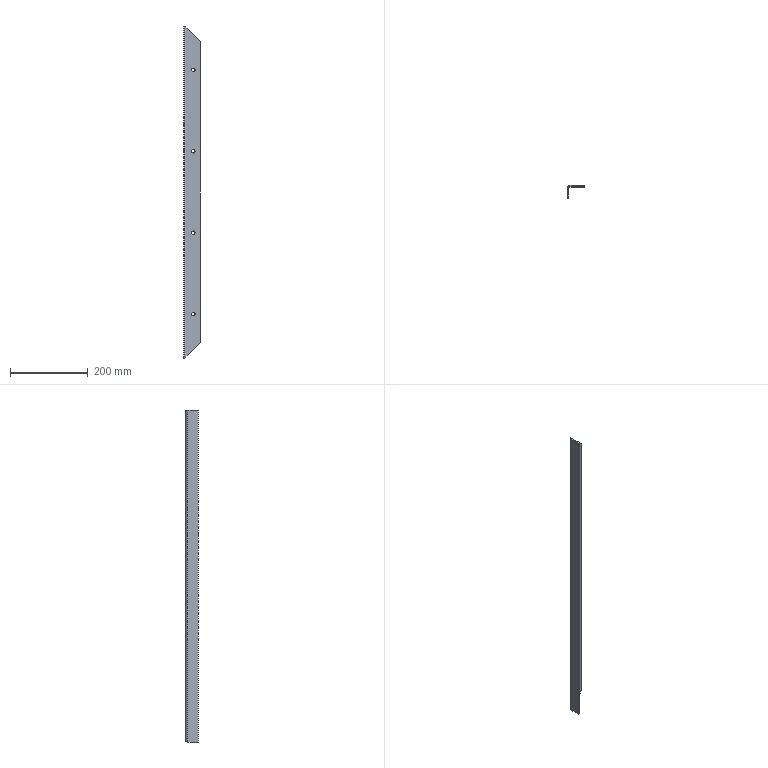Part | STEP file | 750038392 | 1 solid | 22 faces | box 43 x 33 x 856 mm | volume 176921 mm3 | cylinder 10 | plane 10 | spline 2 | commonest cylinder face diameters 9 x8 6 x1 12 x1
STEP:
#1=CARTESIAN_POINT('',(22.,0.,310.5));
#2=VERTEX_POINT('',#1);
#3=CARTESIAN_POINT('',(22.,0.,319.5));
#4=VERTEX_POINT('',#3);
#5=CARTESIAN_POINT('',(22.,0.,315.));
#6=DIRECTION('',(0.,1.,0.));
#7=DIRECTION('',(0.,0.,1.));
#8=AXIS2_PLACEMENT_3D('',#5,#6,#7);
#9=CIRCLE('',#8,4.5);
#10=EDGE_CURVE('',#2,#4,#9,.T.);
#11=ORIENTED_EDGE('',*,*,#10,.F.);
#12=CARTESIAN_POINT('',(22.,3.,310.5));
#13=VERTEX_POINT('',#12);
#14=CARTESIAN_POINT('',(22.,-854.714,310.5));
#15=DIRECTION('',(0.,1.,0.));
#16=VECTOR('',#15,1000.);
#17=LINE('',#14,#16);
#18=EDGE_CURVE('',#2,#13,#17,.T.);
#19=ORIENTED_EDGE('',*,*,#18,.T.);
#20=CARTESIAN_POINT('',(22.,3.,319.5));
#21=VERTEX_POINT('',#20);
#22=CARTESIAN_POINT('',(22.,3.,315.));
#23=DIRECTION('',(0.,1.,0.));
#24=DIRECTION('',(0.,0.,1.));
#25=AXIS2_PLACEMENT_3D('',#22,#23,#24);
#26=CIRCLE('',#25,4.5);
#27=EDGE_CURVE('',#13,#21,#26,.T.);
#28=ORIENTED_EDGE('',*,*,#27,.T.);
#29=CARTESIAN_POINT('',(22.,-854.714,319.5));
#30=DIRECTION('',(0.,1.,0.));
#31=VECTOR('',#30,1000.);
#32=LINE('',#29,#31);
#33=EDGE_CURVE('',#4,#21,#32,.T.);
#34=ORIENTED_EDGE('',*,*,#33,.F.);
#35=EDGE_LOOP('',(#11,#19,#28,#34));
#36=FACE_OUTER_BOUND('',#35,.T.);
#37=CARTESIAN_POINT('',(22.,-854.714,315.));
#38=DIRECTION('',(0.,1.,0.));
#39=DIRECTION('',(0.,0.,1.));
#40=AXIS2_PLACEMENT_3D('',#37,#38,#39);
#41=CYLINDRICAL_SURFACE('',#40,4.5);
#42=ADVANCED_FACE('',(#36),#41,.F.);
#43=CARTESIAN_POINT('',(22.,0.,100.5));
#44=VERTEX_POINT('',#43);
#45=CARTESIAN_POINT('',(22.,0.,109.5));
#46=VERTEX_POINT('',#45);
#47=CARTESIAN_POINT('',(22.,0.,105.));
#48=DIRECTION('',(0.,1.,0.));
#49=DIRECTION('',(0.,0.,1.));
#50=AXIS2_PLACEMENT_3D('',#47,#48,#49);
#51=CIRCLE('',#50,4.5);
#52=EDGE_CURVE('',#44,#46,#51,.T.);
#53=ORIENTED_EDGE('',*,*,#52,.F.);
#54=CARTESIAN_POINT('',(22.,3.,100.5));
#55=VERTEX_POINT('',#54);
#56=CARTESIAN_POINT('',(22.,-854.714,100.5));
#57=DIRECTION('',(0.,1.,0.));
#58=VECTOR('',#57,1000.);
#59=LINE('',#56,#58);
#60=EDGE_CURVE('',#44,#55,#59,.T.);
#61=ORIENTED_EDGE('',*,*,#60,.T.);
#62=CARTESIAN_POINT('',(22.,3.,109.5));
#63=VERTEX_POINT('',#62);
#64=CARTESIAN_POINT('',(22.,3.,105.));
#65=DIRECTION('',(0.,1.,0.));
#66=DIRECTION('',(0.,0.,1.));
#67=AXIS2_PLACEMENT_3D('',#64,#65,#66);
#68=CIRCLE('',#67,4.5);
#69=EDGE_CURVE('',#55,#63,#68,.T.);
#70=ORIENTED_EDGE('',*,*,#69,.T.);
#71=CARTESIAN_POINT('',(22.,-854.714,109.5));
#72=DIRECTION('',(0.,1.,0.));
#73=VECTOR('',#72,1000.);
#74=LINE('',#71,#73);
#75=EDGE_CURVE('',#46,#63,#74,.T.);
#76=ORIENTED_EDGE('',*,*,#75,.F.);
#77=EDGE_LOOP('',(#53,#61,#70,#76));
#78=FACE_OUTER_BOUND('',#77,.T.);
#79=CARTESIAN_POINT('',(22.,-854.714,105.));
#80=DIRECTION('',(0.,1.,0.));
#81=DIRECTION('',(0.,0.,1.));
#82=AXIS2_PLACEMENT_3D('',#79,#80,#81);
#83=CYLINDRICAL_SURFACE('',#82,4.5);
#84=ADVANCED_FACE('',(#78),#83,.F.);
#85=CARTESIAN_POINT('',(22.,0.,-109.5));
#86=VERTEX_POINT('',#85);
#87=CARTESIAN_POINT('',(22.,0.,-100.5));
#88=VERTEX_POINT('',#87);
#89=CARTESIAN_POINT('',(22.,0.,-105.));
#90=DIRECTION('',(0.,1.,0.));
#91=DIRECTION('',(0.,0.,1.));
#92=AXIS2_PLACEMENT_3D('',#89,#90,#91);
#93=CIRCLE('',#92,4.5);
#94=EDGE_CURVE('',#86,#88,#93,.T.);
#95=ORIENTED_EDGE('',*,*,#94,.F.);
#96=CARTESIAN_POINT('',(22.,3.,-109.5));
#97=VERTEX_POINT('',#96);
#98=CARTESIAN_POINT('',(22.,-854.714,-109.5));
#99=DIRECTION('',(0.,1.,0.));
#100=VECTOR('',#99,1000.);
#101=LINE('',#98,#100);
#102=EDGE_CURVE('',#86,#97,#101,.T.);
#103=ORIENTED_EDGE('',*,*,#102,.T.);
#104=CARTESIAN_POINT('',(22.,3.,-100.5));
#105=VERTEX_POINT('',#104);
#106=CARTESIAN_POINT('',(22.,3.,-105.));
#107=DIRECTION('',(0.,1.,0.));
#108=DIRECTION('',(0.,0.,1.));
#109=AXIS2_PLACEMENT_3D('',#106,#107,#108);
#110=CIRCLE('',#109,4.5);
#111=EDGE_CURVE('',#97,#105,#110,.T.);
#112=ORIENTED_EDGE('',*,*,#111,.T.);
#113=CARTESIAN_POINT('',(22.,-854.714,-100.5));
#114=DIRECTION('',(0.,1.,0.));
#115=VECTOR('',#114,1000.);
#116=LINE('',#113,#115);
#117=EDGE_CURVE('',#88,#105,#116,.T.);
#118=ORIENTED_EDGE('',*,*,#117,.F.);
#119=EDGE_LOOP('',(#95,#103,#112,#118));
#120=FACE_OUTER_BOUND('',#119,.T.);
#121=CARTESIAN_POINT('',(22.,-854.714,-105.));
#122=DIRECTION('',(0.,1.,0.));
#123=DIRECTION('',(0.,0.,1.));
#124=AXIS2_PLACEMENT_3D('',#121,#122,#123);
#125=CYLINDRICAL_SURFACE('',#124,4.5);
#126=ADVANCED_FACE('',(#120),#125,.F.);
#127=CARTESIAN_POINT('',(22.,0.,-319.5));
#128=VERTEX_POINT('',#127);
#129=CARTESIAN_POINT('',(22.,0.,-310.5));
#130=VERTEX_POINT('',#129);
#131=CARTESIAN_POINT('',(22.,0.,-315.));
#132=DIRECTION('',(0.,1.,0.));
#133=DIRECTION('',(0.,0.,1.));
#134=AXIS2_PLACEMENT_3D('',#131,#132,#133);
#135=CIRCLE('',#134,4.5);
#136=EDGE_CURVE('',#128,#130,#135,.T.);
#137=ORIENTED_EDGE('',*,*,#136,.F.);
#138=CARTESIAN_POINT('',(22.,3.,-319.5));
#139=VERTEX_POINT('',#138);
#140=CARTESIAN_POINT('',(22.,-854.714,-319.5));
#141=DIRECTION('',(0.,1.,0.));
#142=VECTOR('',#141,1000.);
#143=LINE('',#140,#142);
#144=EDGE_CURVE('',#128,#139,#143,.T.);
#145=ORIENTED_EDGE('',*,*,#144,.T.);
#146=CARTESIAN_POINT('',(22.,3.,-310.5));
#147=VERTEX_POINT('',#146);
#148=CARTESIAN_POINT('',(22.,3.,-315.));
#149=DIRECTION('',(0.,1.,0.));
#150=DIRECTION('',(0.,0.,1.));
#151=AXIS2_PLACEMENT_3D('',#148,#149,#150);
#152=CIRCLE('',#151,4.5);
#153=EDGE_CURVE('',#139,#147,#152,.T.);
#154=ORIENTED_EDGE('',*,*,#153,.T.);
#155=CARTESIAN_POINT('',(22.,-854.714,-310.5));
#156=DIRECTION('',(0.,1.,0.));
#157=VECTOR('',#156,1000.);
#158=LINE('',#155,#157);
#159=EDGE_CURVE('',#130,#147,#158,.T.);
#160=ORIENTED_EDGE('',*,*,#159,.F.);
#161=EDGE_LOOP('',(#137,#145,#154,#160));
#162=FACE_OUTER_BOUND('',#161,.T.);
#163=CARTESIAN_POINT('',(22.,-854.714,-315.));
#164=DIRECTION('',(0.,1.,0.));
#165=DIRECTION('',(0.,0.,1.));
#166=AXIS2_PLACEMENT_3D('',#163,#164,#165);
#167=CYLINDRICAL_SURFACE('',#166,4.5);
#168=ADVANCED_FACE('',(#162),#167,.F.);
#169=CARTESIAN_POINT('',(40.,3.,-388.));
#170=VERTEX_POINT('',#169);
#171=CARTESIAN_POINT('',(40.,3.,388.));
#172=VERTEX_POINT('',#171);
#173=CARTESIAN_POINT('',(40.,3.,428.));
#174=DIRECTION('',(0.,0.,1.));
#175=VECTOR('',#174,1000.);
#176=LINE('',#173,#175);
#177=EDGE_CURVE('',#170,#172,#176,.T.);
#178=ORIENTED_EDGE('',*,*,#177,.F.);
#179=CARTESIAN_POINT('',(3.,3.,-425.));
#180=VERTEX_POINT('',#179);
#181=CARTESIAN_POINT('',(3.,3.,-425.));
#182=DIRECTION('',(0.7071,0.,0.7071));
#183=VECTOR('',#182,1000.);
#184=LINE('',#181,#183);
#185=EDGE_CURVE('',#180,#170,#184,.T.);
#186=ORIENTED_EDGE('',*,*,#185,.F.);
#187=CARTESIAN_POINT('',(3.,3.,425.));
#188=VERTEX_POINT('',#187);
#189=CARTESIAN_POINT('',(3.,3.,428.));
#190=DIRECTION('',(0.,0.,-1.));
#191=VECTOR('',#190,1000.);
#192=LINE('',#189,#191);
#193=EDGE_CURVE('',#188,#180,#192,.T.);
#194=ORIENTED_EDGE('',*,*,#193,.F.);
#195=CARTESIAN_POINT('',(40.,3.,388.));
#196=DIRECTION('',(-0.7071,0.,0.7071));
#197=VECTOR('',#196,1000.);
#198=LINE('',#195,#197);
#199=EDGE_CURVE('',#172,#188,#198,.T.);
#200=ORIENTED_EDGE('',*,*,#199,.F.);
#201=EDGE_LOOP('',(#178,#186,#194,#200));
#202=FACE_OUTER_BOUND('',#201,.T.);
#203=CARTESIAN_POINT('',(22.,3.,315.));
#204=DIRECTION('',(0.,1.,0.));
#205=DIRECTION('',(0.,0.,1.));
#206=AXIS2_PLACEMENT_3D('',#203,#204,#205);
#207=CIRCLE('',#206,4.5);
#208=EDGE_CURVE('',#21,#13,#207,.T.);
#209=ORIENTED_EDGE('',*,*,#208,.F.);
#210=ORIENTED_EDGE('',*,*,#27,.F.);
#211=EDGE_LOOP('',(#209,#210));
#212=FACE_BOUND('',#211,.T.);
#213=CARTESIAN_POINT('',(22.,3.,105.));
#214=DIRECTION('',(0.,1.,0.));
#215=DIRECTION('',(0.,0.,1.));
#216=AXIS2_PLACEMENT_3D('',#213,#214,#215);
#217=CIRCLE('',#216,4.5);
#218=EDGE_CURVE('',#63,#55,#217,.T.);
#219=ORIENTED_EDGE('',*,*,#218,.F.);
#220=ORIENTED_EDGE('',*,*,#69,.F.);
#221=EDGE_LOOP('',(#219,#220));
#222=FACE_BOUND('',#221,.T.);
#223=CARTESIAN_POINT('',(22.,3.,-105.));
#224=DIRECTION('',(0.,1.,0.));
#225=DIRECTION('',(0.,0.,1.));
#226=AXIS2_PLACEMENT_3D('',#223,#224,#225);
#227=CIRCLE('',#226,4.5);
#228=EDGE_CURVE('',#105,#97,#227,.T.);
#229=ORIENTED_EDGE('',*,*,#228,.F.);
#230=ORIENTED_EDGE('',*,*,#111,.F.);
#231=EDGE_LOOP('',(#229,#230));
#232=FACE_BOUND('',#231,.T.);
#233=CARTESIAN_POINT('',(22.,3.,-315.));
#234=DIRECTION('',(0.,1.,0.));
#235=DIRECTION('',(0.,0.,1.));
#236=AXIS2_PLACEMENT_3D('',#233,#234,#235);
#237=CIRCLE('',#236,4.5);
#238=EDGE_CURVE('',#147,#139,#237,.T.);
#239=ORIENTED_EDGE('',*,*,#238,.F.);
#240=ORIENTED_EDGE('',*,*,#153,.F.);
#241=EDGE_LOOP('',(#239,#240));
#242=FACE_BOUND('',#241,.T.);
#243=CARTESIAN_POINT('',(40.,3.,428.));
#244=DIRECTION('',(0.,-1.,0.));
#245=DIRECTION('',(0.,0.,-1.));
#246=AXIS2_PLACEMENT_3D('',#243,#244,#245);
#247=PLANE('',#246);
#248=ADVANCED_FACE('',(#202,#212,#222,#232,#242),#247,.F.);
#249=CARTESIAN_POINT('',(40.,0.,388.));
#250=VERTEX_POINT('',#249);
#251=CARTESIAN_POINT('',(40.,0.,388.));
#252=DIRECTION('',(0.,1.,0.));
#253=VECTOR('',#252,1000.);
#254=LINE('',#251,#253);
#255=EDGE_CURVE('',#250,#172,#254,.T.);
#256=ORIENTED_EDGE('',*,*,#255,.T.);
#257=ORIENTED_EDGE('',*,*,#199,.T.);
#258=CARTESIAN_POINT('',(3.,0.,425.));
#259=VERTEX_POINT('',#258);
#260=CARTESIAN_POINT('',(3.,0.,425.));
#261=DIRECTION('',(0.,-1.,0.));
#262=VECTOR('',#261,1000.);
#263=LINE('',#260,#262);
#264=EDGE_CURVE('',#188,#259,#263,.T.);
#265=ORIENTED_EDGE('',*,*,#264,.T.);
#266=CARTESIAN_POINT('',(20.,0.,408.));
#267=DIRECTION('',(0.7071,0.,-0.7071));
#268=VECTOR('',#267,1000.);
#269=LINE('',#266,#268);
#270=EDGE_CURVE('',#259,#250,#269,.T.);
#271=ORIENTED_EDGE('',*,*,#270,.T.);
#272=EDGE_LOOP('',(#256,#257,#265,#271));
#273=FACE_OUTER_BOUND('',#272,.T.);
#274=CARTESIAN_POINT('',(20.,0.,408.));
#275=DIRECTION('',(0.7071,0.,0.7071));
#276=DIRECTION('',(0.7071,0.,-0.7071));
#277=AXIS2_PLACEMENT_3D('',#274,#275,#276);
#278=PLANE('',#277);
#279=ADVANCED_FACE('',(#273),#278,.T.);
#280=ORIENTED_EDGE('',*,*,#255,.F.);
#281=CARTESIAN_POINT('',(40.,0.,-388.));
#282=VERTEX_POINT('',#281);
#283=CARTESIAN_POINT('',(40.,0.,428.));
#284=DIRECTION('',(0.,0.,1.));
#285=VECTOR('',#284,1000.);
#286=LINE('',#283,#285);
#287=EDGE_CURVE('',#282,#250,#286,.T.);
#288=ORIENTED_EDGE('',*,*,#287,.F.);
#289=CARTESIAN_POINT('',(40.,0.,-388.));
#290=DIRECTION('',(0.,-1.,0.));
#291=VECTOR('',#290,1000.);
#292=LINE('',#289,#291);
#293=EDGE_CURVE('',#170,#282,#292,.T.);
#294=ORIENTED_EDGE('',*,*,#293,.F.);
#295=ORIENTED_EDGE('',*,*,#177,.T.);
#296=EDGE_LOOP('',(#280,#288,#294,#295));
#297=FACE_OUTER_BOUND('',#296,.T.);
#298=CARTESIAN_POINT('',(40.,0.,428.));
#299=DIRECTION('',(-1.,0.,0.));
#300=DIRECTION('',(0.,0.,1.));
#301=AXIS2_PLACEMENT_3D('',#298,#299,#300);
#302=PLANE('',#301);
#303=ADVANCED_FACE('',(#297),#302,.F.);
#304=CARTESIAN_POINT('',(3.,0.,-425.));
#305=VERTEX_POINT('',#304);
#306=CARTESIAN_POINT('',(3.,0.,-425.));
#307=DIRECTION('',(0.,1.,0.));
#308=VECTOR('',#307,1000.);
#309=LINE('',#306,#308);
#310=EDGE_CURVE('',#305,#180,#309,.T.);
#311=ORIENTED_EDGE('',*,*,#310,.T.);
#312=ORIENTED_EDGE('',*,*,#185,.T.);
#313=ORIENTED_EDGE('',*,*,#293,.T.);
#314=CARTESIAN_POINT('',(448.,0.,20.));
#315=DIRECTION('',(-0.7071,0.,-0.7071));
#316=VECTOR('',#315,1000.);
#317=LINE('',#314,#316);
#318=EDGE_CURVE('',#282,#305,#317,.T.);
#319=ORIENTED_EDGE('',*,*,#318,.T.);
#320=EDGE_LOOP('',(#311,#312,#313,#319));
#321=FACE_OUTER_BOUND('',#320,.T.);
#322=CARTESIAN_POINT('',(448.,0.,20.));
#323=DIRECTION('',(0.7071,0.,-0.7071));
#324=DIRECTION('',(-0.7071,0.,-0.7071));
#325=AXIS2_PLACEMENT_3D('',#322,#323,#324);
#326=PLANE('',#325);
#327=ADVANCED_FACE('',(#321),#326,.T.);
#328=CARTESIAN_POINT('',(-3.,-3.,-428.));
#329=VERTEX_POINT('',#328);
#330=CARTESIAN_POINT('',(3.,3.,-425.));
#331=CARTESIAN_POINT('',(-1.,3.,-427.));
#332=CARTESIAN_POINT('',(-3.,0.,-428.));
#333=CARTESIAN_POINT('',(-3.,-3.,-428.));
#334=(BOUNDED_CURVE()B_SPLINE_CURVE(3,(#330,#331,#332,#333),.UNSPECIFIED.,.F.,.F.)B_SPLINE_CURVE_WITH_KNOTS((4,4),(0.,0.009933),.UNSPECIFIED.)CURVE()GEOMETRIC_REPRESENTATION_ITEM()RATIONAL_B_SPLINE_CURVE((0.5,0.5,0.6667,1.))REPRESENTATION_ITEM(''));
#335=EDGE_CURVE('',#180,#329,#334,.T.);
#336=ORIENTED_EDGE('',*,*,#335,.T.);
#337=CARTESIAN_POINT('',(-3.,-3.,428.));
#338=VERTEX_POINT('',#337);
#339=CARTESIAN_POINT('',(-3.,-3.,428.));
#340=DIRECTION('',(0.,0.,1.));
#341=VECTOR('',#340,1000.);
#342=LINE('',#339,#341);
#343=EDGE_CURVE('',#329,#338,#342,.T.);
#344=ORIENTED_EDGE('',*,*,#343,.T.);
#345=CARTESIAN_POINT('',(-3.,-3.,428.));
#346=CARTESIAN_POINT('',(-3.,0.,428.));
#347=CARTESIAN_POINT('',(-1.,3.,427.));
#348=CARTESIAN_POINT('',(3.,3.,425.));
#349=(BOUNDED_CURVE()B_SPLINE_CURVE(3,(#345,#346,#347,#348),.UNSPECIFIED.,.F.,.T.)B_SPLINE_CURVE_WITH_KNOTS((4,4),(0.,0.009979),.UNSPECIFIED.)CURVE()GEOMETRIC_REPRESENTATION_ITEM()RATIONAL_B_SPLINE_CURVE((1.,0.6667,0.5,0.5))REPRESENTATION_ITEM(''));
#350=EDGE_CURVE('',#338,#188,#349,.T.);
#351=ORIENTED_EDGE('',*,*,#350,.T.);
#352=ORIENTED_EDGE('',*,*,#193,.T.);
#353=EDGE_LOOP('',(#336,#344,#351,#352));
#354=FACE_OUTER_BOUND('',#353,.T.);
#355=CARTESIAN_POINT('',(3.,-3.,428.));
#356=DIRECTION('',(0.,0.,-1.));
#357=DIRECTION('',(-1.,0.,0.));
#358=AXIS2_PLACEMENT_3D('',#355,#356,#357);
#359=CYLINDRICAL_SURFACE('',#358,6.);
#360=ADVANCED_FACE('',(#354),#359,.T.);
#361=ORIENTED_EDGE('',*,*,#18,.F.);
#362=CARTESIAN_POINT('',(22.,0.,315.));
#363=DIRECTION('',(0.,1.,0.));
#364=DIRECTION('',(0.,0.,1.));
#365=AXIS2_PLACEMENT_3D('',#362,#363,#364);
#366=CIRCLE('',#365,4.5);
#367=EDGE_CURVE('',#4,#2,#366,.T.);
#368=ORIENTED_EDGE('',*,*,#367,.F.);
#369=ORIENTED_EDGE('',*,*,#33,.T.);
#370=ORIENTED_EDGE('',*,*,#208,.T.);
#371=EDGE_LOOP('',(#361,#368,#369,#370));
#372=FACE_OUTER_BOUND('',#371,.T.);
#373=CARTESIAN_POINT('',(22.,-854.714,315.));
#374=DIRECTION('',(0.,1.,0.));
#375=DIRECTION('',(0.,0.,1.));
#376=AXIS2_PLACEMENT_3D('',#373,#374,#375);
#377=CYLINDRICAL_SURFACE('',#376,4.5);
#378=ADVANCED_FACE('',(#372),#377,.F.);
#379=ORIENTED_EDGE('',*,*,#60,.F.);
#380=CARTESIAN_POINT('',(22.,0.,105.));
#381=DIRECTION('',(0.,1.,0.));
#382=DIRECTION('',(0.,0.,1.));
#383=AXIS2_PLACEMENT_3D('',#380,#381,#382);
#384=CIRCLE('',#383,4.5);
#385=EDGE_CURVE('',#46,#44,#384,.T.);
#386=ORIENTED_EDGE('',*,*,#385,.F.);
#387=ORIENTED_EDGE('',*,*,#75,.T.);
#388=ORIENTED_EDGE('',*,*,#218,.T.);
#389=EDGE_LOOP('',(#379,#386,#387,#388));
#390=FACE_OUTER_BOUND('',#389,.T.);
#391=CARTESIAN_POINT('',(22.,-854.714,105.));
#392=DIRECTION('',(0.,1.,0.));
#393=DIRECTION('',(0.,0.,1.));
#394=AXIS2_PLACEMENT_3D('',#391,#392,#393);
#395=CYLINDRICAL_SURFACE('',#394,4.5);
#396=ADVANCED_FACE('',(#390),#395,.F.);
#397=ORIENTED_EDGE('',*,*,#102,.F.);
#398=CARTESIAN_POINT('',(22.,0.,-105.));
#399=DIRECTION('',(0.,1.,0.));
#400=DIRECTION('',(0.,0.,1.));
#401=AXIS2_PLACEMENT_3D('',#398,#399,#400);
#402=CIRCLE('',#401,4.5);
#403=EDGE_CURVE('',#88,#86,#402,.T.);
#404=ORIENTED_EDGE('',*,*,#403,.F.);
#405=ORIENTED_EDGE('',*,*,#117,.T.);
#406=ORIENTED_EDGE('',*,*,#228,.T.);
#407=EDGE_LOOP('',(#397,#404,#405,#406));
#408=FACE_OUTER_BOUND('',#407,.T.);
#409=CARTESIAN_POINT('',(22.,-854.714,-105.));
#410=DIRECTION('',(0.,1.,0.));
#411=DIRECTION('',(0.,0.,1.));
#412=AXIS2_PLACEMENT_3D('',#409,#410,#411);
#413=CYLINDRICAL_SURFACE('',#412,4.5);
#414=ADVANCED_FACE('',(#408),#413,.F.);
#415=ORIENTED_EDGE('',*,*,#144,.F.);
#416=CARTESIAN_POINT('',(22.,0.,-315.));
#417=DIRECTION('',(0.,1.,0.));
#418=DIRECTION('',(0.,0.,1.));
#419=AXIS2_PLACEMENT_3D('',#416,#417,#418);
#420=CIRCLE('',#419,4.5);
#421=EDGE_CURVE('',#130,#128,#420,.T.);
#422=ORIENTED_EDGE('',*,*,#421,.F.);
#423=ORIENTED_EDGE('',*,*,#159,.T.);
#424=ORIENTED_EDGE('',*,*,#238,.T.);
#425=EDGE_LOOP('',(#415,#422,#423,#424));
#426=FACE_OUTER_BOUND('',#425,.T.);
#427=CARTESIAN_POINT('',(22.,-854.714,-315.));
#428=DIRECTION('',(0.,1.,0.));
#429=DIRECTION('',(0.,0.,1.));
#430=AXIS2_PLACEMENT_3D('',#427,#428,#429);
#431=CYLINDRICAL_SURFACE('',#430,4.5);
#432=ADVANCED_FACE('',(#426),#431,.F.);
#433=CARTESIAN_POINT('',(3.,0.,428.));
#434=DIRECTION('',(0.,0.,-1.));
#435=VECTOR('',#434,1000.);
#436=LINE('',#433,#435);
#437=EDGE_CURVE('',#259,#305,#436,.T.);
#438=ORIENTED_EDGE('',*,*,#437,.T.);
#439=ORIENTED_EDGE('',*,*,#318,.F.);
#440=ORIENTED_EDGE('',*,*,#287,.T.);
#441=ORIENTED_EDGE('',*,*,#270,.F.);
#442=EDGE_LOOP('',(#438,#439,#440,#441));
#443=FACE_OUTER_BOUND('',#442,.T.);
#444=ORIENTED_EDGE('',*,*,#367,.T.);
#445=ORIENTED_EDGE('',*,*,#10,.T.);
#446=EDGE_LOOP('',(#444,#445));
#447=FACE_BOUND('',#446,.T.);
#448=ORIENTED_EDGE('',*,*,#385,.T.);
#449=ORIENTED_EDGE('',*,*,#52,.T.);
#450=EDGE_LOOP('',(#448,#449));
#451=FACE_BOUND('',#450,.T.);
#452=ORIENTED_EDGE('',*,*,#403,.T.);
#453=ORIENTED_EDGE('',*,*,#94,.T.);
#454=EDGE_LOOP('',(#452,#453));
#455=FACE_BOUND('',#454,.T.);
#456=ORIENTED_EDGE('',*,*,#421,.T.);
#457=ORIENTED_EDGE('',*,*,#136,.T.);
#458=EDGE_LOOP('',(#456,#457));
#459=FACE_BOUND('',#458,.T.);
#460=CARTESIAN_POINT('',(40.,0.,428.));
#461=DIRECTION('',(0.,-1.,0.));
#462=DIRECTION('',(0.,0.,-1.));
#463=AXIS2_PLACEMENT_3D('',#460,#461,#462);
#464=PLANE('',#463);
#465=ADVANCED_FACE('',(#443,#447,#451,#455,#459),#464,.T.);
#466=CARTESIAN_POINT('',(0.,-3.,428.));
#467=VERTEX_POINT('',#466);
#468=CARTESIAN_POINT('',(3.,0.,425.));
#469=CARTESIAN_POINT('',(1.,0.,427.));
#470=CARTESIAN_POINT('',(0.,-1.5,428.));
#471=CARTESIAN_POINT('',(0.,-3.,428.));
#472=(BOUNDED_CURVE()B_SPLINE_CURVE(3,(#468,#469,#470,#471),.UNSPECIFIED.,.F.,.T.)B_SPLINE_CURVE_WITH_KNOTS((4,4),(0.,0.005677),.UNSPECIFIED.)CURVE()GEOMETRIC_REPRESENTATION_ITEM()RATIONAL_B_SPLINE_CURVE((0.5,0.5,0.6667,1.))REPRESENTATION_ITEM(''));
#473=EDGE_CURVE('',#259,#467,#472,.T.);
#474=ORIENTED_EDGE('',*,*,#473,.F.);
#475=ORIENTED_EDGE('',*,*,#264,.F.);
#476=ORIENTED_EDGE('',*,*,#350,.F.);
#477=CARTESIAN_POINT('',(-1.5,-3.,428.));
#478=DIRECTION('',(-1.,0.,0.));
#479=VECTOR('',#478,1000.);
#480=LINE('',#477,#479);
#481=EDGE_CURVE('',#467,#338,#480,.T.);
#482=ORIENTED_EDGE('',*,*,#481,.F.);
#483=EDGE_LOOP('',(#474,#475,#476,#482));
#484=FACE_OUTER_BOUND('',#483,.T.);
#485=CARTESIAN_POINT('',(6.,-3.,422.));
#486=CARTESIAN_POINT('',(7.,-3.,422.));
#487=CARTESIAN_POINT('',(8.,-3.,422.));
#488=CARTESIAN_POINT('',(9.,-3.,422.));
#489=CARTESIAN_POINT('',(6.,3.,422.));
#490=CARTESIAN_POINT('',(7.,5.,422.));
#491=CARTESIAN_POINT('',(8.,7.,422.));
#492=CARTESIAN_POINT('',(9.,9.,422.));
#493=CARTESIAN_POINT('',(0.,3.,428.));
#494=CARTESIAN_POINT('',(-1.,5.,428.));
#495=CARTESIAN_POINT('',(-2.,7.,428.));
#496=CARTESIAN_POINT('',(-3.,9.,428.));
#497=CARTESIAN_POINT('',(0.,-3.,428.));
#498=CARTESIAN_POINT('',(-1.,-3.,428.));
#499=CARTESIAN_POINT('',(-2.,-3.,428.));
#500=CARTESIAN_POINT('',(-3.,-3.,428.));
#501=CARTESIAN_POINT('',(0.,-9.,428.));
#502=CARTESIAN_POINT('',(-1.,-11.,428.));
#503=CARTESIAN_POINT('',(-2.,-13.,428.));
#504=CARTESIAN_POINT('',(-3.,-15.,428.));
#505=CARTESIAN_POINT('',(6.,-9.,422.));
#506=CARTESIAN_POINT('',(7.,-11.,422.));
#507=CARTESIAN_POINT('',(8.,-13.,422.));
#508=CARTESIAN_POINT('',(9.,-15.,422.));
#509=CARTESIAN_POINT('',(6.,-3.,422.));
#510=CARTESIAN_POINT('',(7.,-3.,422.));
#511=CARTESIAN_POINT('',(8.,-3.,422.));
#512=CARTESIAN_POINT('',(9.,-3.,422.));
#513=(BOUNDED_SURFACE()B_SPLINE_SURFACE(3,3,((#485,#486,#487,#488),(#489,#490,#491,#492),(#493,#494,#495,#496),(#497,#498,#499,#500),(#501,#502,#503,#504),(#505,#506,#507,#508),(#509,#510,#511,#512)),.UNSPECIFIED.,.T.,.F.,.F.)B_SPLINE_SURFACE_WITH_KNOTS((4,3,4),(4,4),(0.,0.5,1.),(0.,1.),.UNSPECIFIED.)GEOMETRIC_REPRESENTATION_ITEM()RATIONAL_B_SPLINE_SURFACE(((1.,1.,1.,1.),(0.3333,0.3333,0.3333,0.3333),(0.3333,0.3333,0.3333,0.3333),(1.,1.,1.,1.),(0.3333,0.3333,0.3333,0.3333),(0.3333,0.3333,0.3333,0.3333),(1.,1.,1.,1.)))REPRESENTATION_ITEM('')SURFACE());
#514=ADVANCED_FACE('',(#484),#513,.F.);
#515=CARTESIAN_POINT('',(0.,-3.,-428.));
#516=VERTEX_POINT('',#515);
#517=CARTESIAN_POINT('',(0.,-3.,-428.));
#518=CARTESIAN_POINT('',(0.,-1.5,-428.));
#519=CARTESIAN_POINT('',(1.,0.,-427.));
#520=CARTESIAN_POINT('',(3.,0.,-425.));
#521=(BOUNDED_CURVE()B_SPLINE_CURVE(3,(#517,#518,#519,#520),.UNSPECIFIED.,.F.,.T.)B_SPLINE_CURVE_WITH_KNOTS((4,4),(0.,0.005708),.UNSPECIFIED.)CURVE()GEOMETRIC_REPRESENTATION_ITEM()RATIONAL_B_SPLINE_CURVE((1.,0.6667,0.5,0.5))REPRESENTATION_ITEM(''));
#522=EDGE_CURVE('',#516,#305,#521,.T.);
#523=ORIENTED_EDGE('',*,*,#522,.F.);
#524=CARTESIAN_POINT('',(-1.5,-3.,-428.));
#525=DIRECTION('',(1.,0.,0.));
#526=VECTOR('',#525,1000.);
#527=LINE('',#524,#526);
#528=EDGE_CURVE('',#329,#516,#527,.T.);
#529=ORIENTED_EDGE('',*,*,#528,.F.);
#530=ORIENTED_EDGE('',*,*,#335,.F.);
#531=ORIENTED_EDGE('',*,*,#310,.F.);
#532=EDGE_LOOP('',(#523,#529,#530,#531));
#533=FACE_OUTER_BOUND('',#532,.T.);
#534=CARTESIAN_POINT('',(0.,-3.,-428.));
#535=CARTESIAN_POINT('',(-1.,-3.,-428.));
#536=CARTESIAN_POINT('',(-2.,-3.,-428.));
#537=CARTESIAN_POINT('',(-3.,-3.,-428.));
#538=CARTESIAN_POINT('',(0.,3.,-428.));
#539=CARTESIAN_POINT('',(-1.,5.,-428.));
#540=CARTESIAN_POINT('',(-2.,7.,-428.));
#541=CARTESIAN_POINT('',(-3.,9.,-428.));
#542=CARTESIAN_POINT('',(6.,3.,-422.));
#543=CARTESIAN_POINT('',(7.,5.,-422.));
#544=CARTESIAN_POINT('',(8.,7.,-422.));
#545=CARTESIAN_POINT('',(9.,9.,-422.));
#546=CARTESIAN_POINT('',(6.,-3.,-422.));
#547=CARTESIAN_POINT('',(7.,-3.,-422.));
#548=CARTESIAN_POINT('',(8.,-3.,-422.));
#549=CARTESIAN_POINT('',(9.,-3.,-422.));
#550=CARTESIAN_POINT('',(6.,-9.,-422.));
#551=CARTESIAN_POINT('',(7.,-11.,-422.));
#552=CARTESIAN_POINT('',(8.,-13.,-422.));
#553=CARTESIAN_POINT('',(9.,-15.,-422.));
#554=CARTESIAN_POINT('',(0.,-9.,-428.));
#555=CARTESIAN_POINT('',(-1.,-11.,-428.));
#556=CARTESIAN_POINT('',(-2.,-13.,-428.));
#557=CARTESIAN_POINT('',(-3.,-15.,-428.));
#558=CARTESIAN_POINT('',(0.,-3.,-428.));
#559=CARTESIAN_POINT('',(-1.,-3.,-428.));
#560=CARTESIAN_POINT('',(-2.,-3.,-428.));
#561=CARTESIAN_POINT('',(-3.,-3.,-428.));
#562=(BOUNDED_SURFACE()B_SPLINE_SURFACE(3,3,((#534,#535,#536,#537),(#538,#539,#540,#541),(#542,#543,#544,#545),(#546,#547,#548,#549),(#550,#551,#552,#553),(#554,#555,#556,#557),(#558,#559,#560,#561)),.UNSPECIFIED.,.T.,.F.,.T.)B_SPLINE_SURFACE_WITH_KNOTS((4,3,4),(4,4),(0.,0.5,1.),(0.,1.),.UNSPECIFIED.)GEOMETRIC_REPRESENTATION_ITEM()RATIONAL_B_SPLINE_SURFACE(((1.,1.,1.,1.),(0.3333,0.3333,0.3333,0.3333),(0.3333,0.3333,0.3333,0.3333),(1.,1.,1.,1.),(0.3333,0.3333,0.3333,0.3333),(0.3333,0.3333,0.3333,0.3333),(1.,1.,1.,1.)))REPRESENTATION_ITEM('')SURFACE());
#563=ADVANCED_FACE('',(#533),#562,.F.);
#564=CARTESIAN_POINT('',(-3.,-30.,428.));
#565=VERTEX_POINT('',#564);
#566=CARTESIAN_POINT('',(-3.,-30.,-428.));
#567=VERTEX_POINT('',#566);
#568=CARTESIAN_POINT('',(-3.,-30.,428.));
#569=DIRECTION('',(0.,0.,-1.));
#570=VECTOR('',#569,1000.);
#571=LINE('',#568,#570);
#572=EDGE_CURVE('',#565,#567,#571,.T.);
#573=ORIENTED_EDGE('',*,*,#572,.F.);
#574=CARTESIAN_POINT('',(-3.,0.,428.));
#575=DIRECTION('',(0.,-1.,0.));
#576=VECTOR('',#575,1000.);
#577=LINE('',#574,#576);
#578=EDGE_CURVE('',#338,#565,#577,.T.);
#579=ORIENTED_EDGE('',*,*,#578,.F.);
#580=ORIENTED_EDGE('',*,*,#343,.F.);
#581=CARTESIAN_POINT('',(-3.,0.,-428.));
#582=DIRECTION('',(0.,1.,0.));
#583=VECTOR('',#582,1000.);
#584=LINE('',#581,#583);
#585=EDGE_CURVE('',#567,#329,#584,.T.);
#586=ORIENTED_EDGE('',*,*,#585,.F.);
#587=EDGE_LOOP('',(#573,#579,#580,#586));
#588=FACE_OUTER_BOUND('',#587,.T.);
#589=CARTESIAN_POINT('',(-3.,0.,428.));
#590=DIRECTION('',(1.,0.,0.));
#591=DIRECTION('',(0.,1.,0.));
#592=AXIS2_PLACEMENT_3D('',#589,#590,#591);
#593=PLANE('',#592);
#594=ADVANCED_FACE('',(#588),#593,.F.);
#595=ORIENTED_EDGE('',*,*,#473,.T.);
#596=CARTESIAN_POINT('',(0.,-3.,428.));
#597=DIRECTION('',(0.,0.,1.));
#598=VECTOR('',#597,1000.);
#599=LINE('',#596,#598);
#600=EDGE_CURVE('',#516,#467,#599,.T.);
#601=ORIENTED_EDGE('',*,*,#600,.F.);
#602=ORIENTED_EDGE('',*,*,#522,.T.);
#603=ORIENTED_EDGE('',*,*,#437,.F.);
#604=EDGE_LOOP('',(#595,#601,#602,#603));
#605=FACE_OUTER_BOUND('',#604,.T.);
#606=CARTESIAN_POINT('',(3.,-3.,428.));
#607=DIRECTION('',(0.,0.,-1.));
#608=DIRECTION('',(-1.,0.,0.));
#609=AXIS2_PLACEMENT_3D('',#606,#607,#608);
#610=CYLINDRICAL_SURFACE('',#609,3.);
#611=ADVANCED_FACE('',(#605),#610,.F.);
#612=CARTESIAN_POINT('',(0.,-30.,428.));
#613=VERTEX_POINT('',#612);
#614=CARTESIAN_POINT('',(0.,-30.,428.));
#615=DIRECTION('',(1.,0.,0.));
#616=VECTOR('',#615,1000.);
#617=LINE('',#614,#616);
#618=EDGE_CURVE('',#565,#613,#617,.T.);
#619=ORIENTED_EDGE('',*,*,#618,.T.);
#620=CARTESIAN_POINT('',(0.,0.,428.));
#621=DIRECTION('',(0.,1.,0.));
#622=VECTOR('',#621,1000.);
#623=LINE('',#620,#622);
#624=EDGE_CURVE('',#613,#467,#623,.T.);
#625=ORIENTED_EDGE('',*,*,#624,.T.);
#626=ORIENTED_EDGE('',*,*,#481,.T.);
#627=ORIENTED_EDGE('',*,*,#578,.T.);
#628=EDGE_LOOP('',(#619,#625,#626,#627));
#629=FACE_OUTER_BOUND('',#628,.T.);
#630=CARTESIAN_POINT('',(0.,0.,428.));
#631=DIRECTION('',(0.,0.,1.));
#632=DIRECTION('',(1.,0.,0.));
#633=AXIS2_PLACEMENT_3D('',#630,#631,#632);
#634=PLANE('',#633);
#635=ADVANCED_FACE('',(#629),#634,.T.);
#636=ORIENTED_EDGE('',*,*,#528,.T.);
#637=CARTESIAN_POINT('',(0.,-30.,-428.));
#638=VERTEX_POINT('',#637);
#639=CARTESIAN_POINT('',(0.,0.,-428.));
#640=DIRECTION('',(0.,1.,0.));
#641=VECTOR('',#640,1000.);
#642=LINE('',#639,#641);
#643=EDGE_CURVE('',#638,#516,#642,.T.);
#644=ORIENTED_EDGE('',*,*,#643,.F.);
#645=CARTESIAN_POINT('',(40.,-30.,-428.));
#646=DIRECTION('',(1.,0.,0.));
#647=VECTOR('',#646,1000.);
#648=LINE('',#645,#647);
#649=EDGE_CURVE('',#567,#638,#648,.T.);
#650=ORIENTED_EDGE('',*,*,#649,.F.);
#651=ORIENTED_EDGE('',*,*,#585,.T.);
#652=EDGE_LOOP('',(#636,#644,#650,#651));
#653=FACE_OUTER_BOUND('',#652,.T.);
#654=CARTESIAN_POINT('',(40.,0.,-428.));
#655=DIRECTION('',(0.,0.,1.));
#656=DIRECTION('',(1.,0.,0.));
#657=AXIS2_PLACEMENT_3D('',#654,#655,#656);
#658=PLANE('',#657);
#659=ADVANCED_FACE('',(#653),#658,.F.);
#660=ORIENTED_EDGE('',*,*,#649,.T.);
#661=CARTESIAN_POINT('',(0.,-30.,428.));
#662=DIRECTION('',(0.,0.,1.));
#663=VECTOR('',#662,1000.);
#664=LINE('',#661,#663);
#665=EDGE_CURVE('',#638,#613,#664,.T.);
#666=ORIENTED_EDGE('',*,*,#665,.T.);
#667=ORIENTED_EDGE('',*,*,#618,.F.);
#668=ORIENTED_EDGE('',*,*,#572,.T.);
#669=EDGE_LOOP('',(#660,#666,#667,#668));
#670=FACE_OUTER_BOUND('',#669,.T.);
#671=CARTESIAN_POINT('',(0.,-30.,428.));
#672=DIRECTION('',(0.,-1.,0.));
#673=DIRECTION('',(1.,0.,0.));
#674=AXIS2_PLACEMENT_3D('',#671,#672,#673);
#675=PLANE('',#674);
#676=ADVANCED_FACE('',(#670),#675,.T.);
#677=ORIENTED_EDGE('',*,*,#624,.F.);
#678=ORIENTED_EDGE('',*,*,#665,.F.);
#679=ORIENTED_EDGE('',*,*,#643,.T.);
#680=ORIENTED_EDGE('',*,*,#600,.T.);
#681=EDGE_LOOP('',(#677,#678,#679,#680));
#682=FACE_OUTER_BOUND('',#681,.T.);
#683=CARTESIAN_POINT('',(0.,0.,428.));
#684=DIRECTION('',(1.,0.,0.));
#685=DIRECTION('',(0.,1.,0.));
#686=AXIS2_PLACEMENT_3D('',#683,#684,#685);
#687=PLANE('',#686);
#688=ADVANCED_FACE('',(#682),#687,.T.);
#689=CLOSED_SHELL('',(#42,#84,#126,#168,#248,#279,#303,#327,#360,#378,#396,#414,#432,#465,#514,#563,#594,#611,#635,#659,#676,#688));
#690=MANIFOLD_SOLID_BREP('',#689);
#691=CARTESIAN_POINT('',(0.,0.,0.));
#692=DIRECTION('',(0.,0.,1.));
#693=DIRECTION('',(1.,0.,0.));
#694=AXIS2_PLACEMENT_3D('',#691,#692,#693);
#695=(LENGTH_UNIT()NAMED_UNIT(*)SI_UNIT(.MILLI.,.METRE.));
#696=UNCERTAINTY_MEASURE_WITH_UNIT(LENGTH_MEASURE(0.00001),#695,'','');
#697=(NAMED_UNIT(*)PLANE_ANGLE_UNIT()SI_UNIT($,.RADIAN.));
#698=(NAMED_UNIT(*)SI_UNIT($,.STERADIAN.)SOLID_ANGLE_UNIT());
#699=(GEOMETRIC_REPRESENTATION_CONTEXT(3)GLOBAL_UNCERTAINTY_ASSIGNED_CONTEXT((#696))GLOBAL_UNIT_ASSIGNED_CONTEXT((#695,#697,#698))REPRESENTATION_CONTEXT('',''));
#700=ADVANCED_BREP_SHAPE_REPRESENTATION('',(#690,#694),#699);